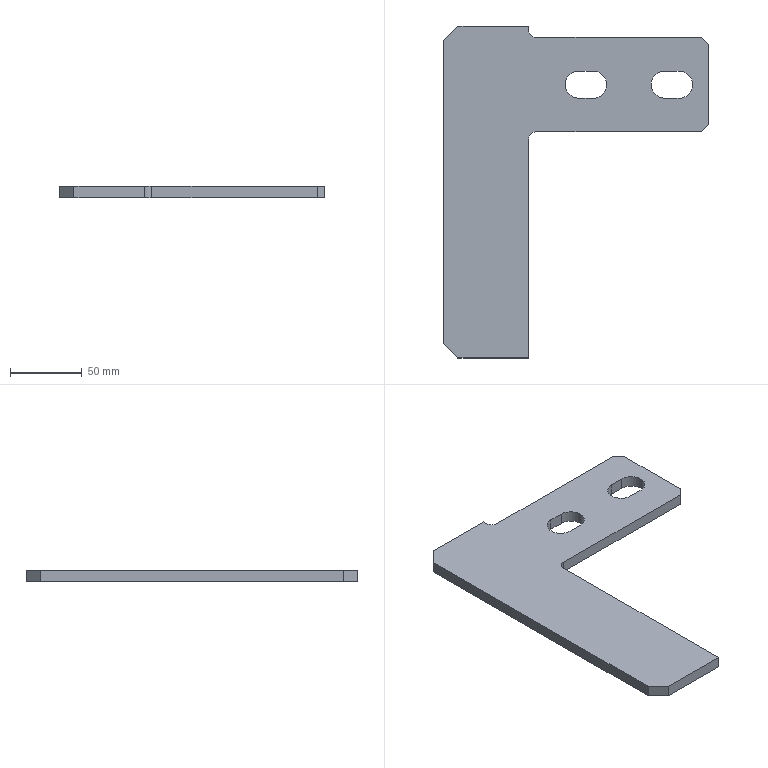Part | STEP file | 筋Plate-250×125-100 | 1 solid | 26 faces | box 185 x 232 x 8 mm | volume 168205 mm3 | plane 18 | cylinder 8 | commonest cylinder face diameters 19 x6 10 x2